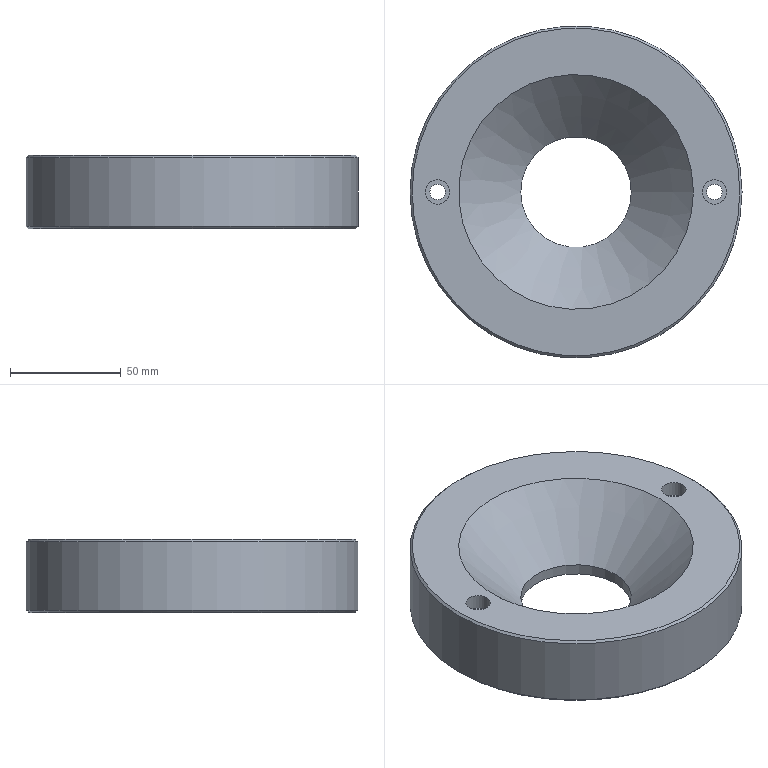Part | STEP file | 车灯-后视镜_id298_x_t | 1 solid | 13 faces | box 149.9 x 149.9 x 33 mm | volume 429222 mm3 | cylinder 6 | plane 4 | cone 3 | commonest cylinder face diameters 7 x2 11 x2 50 x1 149.9 x1
STEP:
#1=CARTESIAN_POINT('',(31.,-25.,243.5));
#2=VERTEX_POINT('',#1);
#3=CARTESIAN_POINT('',(-22.,-25.,243.5));
#4=DIRECTION('',(0.,0.,-1.));
#5=DIRECTION('',(1.,0.,0.));
#6=AXIS2_PLACEMENT_3D('',#3,#4,#5);
#7=CIRCLE('',#6,53.);
#8=EDGE_CURVE('',#2,#2,#7,.T.);
#9=ORIENTED_EDGE('',*,*,#8,.T.);
#10=EDGE_LOOP('',(#9));
#11=FACE_BOUND('',#10,.T.);
#12=CARTESIAN_POINT('',(51.95,-25.,243.5));
#13=VERTEX_POINT('',#12);
#14=CARTESIAN_POINT('',(-22.,-25.,243.5));
#15=DIRECTION('',(0.,0.,1.));
#16=DIRECTION('',(1.,0.,0.));
#17=AXIS2_PLACEMENT_3D('',#14,#15,#16);
#18=CIRCLE('',#17,73.95);
#19=EDGE_CURVE('',#13,#13,#18,.T.);
#20=ORIENTED_EDGE('',*,*,#19,.T.);
#21=EDGE_LOOP('',(#20));
#22=FACE_BOUND('',#21,.T.);
#23=CARTESIAN_POINT('',(46.,-25.,243.5));
#24=VERTEX_POINT('',#23);
#25=CARTESIAN_POINT('',(40.5,-25.,243.5));
#26=DIRECTION('',(0.,0.,1.));
#27=DIRECTION('',(1.,0.,0.));
#28=AXIS2_PLACEMENT_3D('',#25,#26,#27);
#29=CIRCLE('',#28,5.5);
#30=EDGE_CURVE('',#24,#24,#29,.T.);
#31=ORIENTED_EDGE('',*,*,#30,.F.);
#32=EDGE_LOOP('',(#31));
#33=FACE_BOUND('',#32,.T.);
#34=CARTESIAN_POINT('',(-79.,-25.,243.5));
#35=VERTEX_POINT('',#34);
#36=CARTESIAN_POINT('',(-84.5,-25.,243.5));
#37=DIRECTION('',(0.,0.,-1.));
#38=DIRECTION('',(1.,0.,0.));
#39=AXIS2_PLACEMENT_3D('',#36,#37,#38);
#40=CIRCLE('',#39,5.5);
#41=EDGE_CURVE('',#35,#35,#40,.T.);
#42=ORIENTED_EDGE('',*,*,#41,.T.);
#43=EDGE_LOOP('',(#42));
#44=FACE_BOUND('',#43,.T.);
#45=CARTESIAN_POINT('',(-22.,-25.,243.5));
#46=DIRECTION('',(0.,0.,1.));
#47=DIRECTION('',(0.,1.,0.));
#48=AXIS2_PLACEMENT_3D('',#45,#46,#47);
#49=PLANE('',#48);
#50=ADVANCED_FACE('',(#11,#22,#33,#44),#49,.T.);
#51=CARTESIAN_POINT('',(-95.95,-25.,210.5));
#52=VERTEX_POINT('',#51);
#53=CARTESIAN_POINT('',(-22.,-25.,210.5));
#54=DIRECTION('',(0.,0.,-1.));
#55=DIRECTION('',(-1.,0.,0.));
#56=AXIS2_PLACEMENT_3D('',#53,#54,#55);
#57=CIRCLE('',#56,73.95);
#58=EDGE_CURVE('',#52,#52,#57,.T.);
#59=ORIENTED_EDGE('',*,*,#58,.T.);
#60=EDGE_LOOP('',(#59));
#61=FACE_BOUND('',#60,.T.);
#62=CARTESIAN_POINT('',(37.,-25.,210.5));
#63=VERTEX_POINT('',#62);
#64=CARTESIAN_POINT('',(40.5,-25.,210.5));
#65=DIRECTION('',(0.,0.,-1.));
#66=DIRECTION('',(-1.,0.,0.));
#67=AXIS2_PLACEMENT_3D('',#64,#65,#66);
#68=CIRCLE('',#67,3.5);
#69=EDGE_CURVE('',#63,#63,#68,.T.);
#70=ORIENTED_EDGE('',*,*,#69,.F.);
#71=EDGE_LOOP('',(#70));
#72=FACE_BOUND('',#71,.T.);
#73=CARTESIAN_POINT('',(-88.,-25.,210.5));
#74=VERTEX_POINT('',#73);
#75=CARTESIAN_POINT('',(-84.5,-25.,210.5));
#76=DIRECTION('',(0.,0.,-1.));
#77=DIRECTION('',(-1.,0.,0.));
#78=AXIS2_PLACEMENT_3D('',#75,#76,#77);
#79=CIRCLE('',#78,3.5);
#80=EDGE_CURVE('',#74,#74,#79,.T.);
#81=ORIENTED_EDGE('',*,*,#80,.F.);
#82=EDGE_LOOP('',(#81));
#83=FACE_BOUND('',#82,.T.);
#84=CARTESIAN_POINT('',(-47.,-25.,210.5));
#85=VERTEX_POINT('',#84);
#86=CARTESIAN_POINT('',(-22.,-25.,210.5));
#87=DIRECTION('',(0.,0.,-1.));
#88=DIRECTION('',(-1.,0.,0.));
#89=AXIS2_PLACEMENT_3D('',#86,#87,#88);
#90=CIRCLE('',#89,25.);
#91=EDGE_CURVE('',#85,#85,#90,.T.);
#92=ORIENTED_EDGE('',*,*,#91,.F.);
#93=EDGE_LOOP('',(#92));
#94=FACE_BOUND('',#93,.T.);
#95=CARTESIAN_POINT('',(-22.,-25.,210.5));
#96=DIRECTION('',(0.,0.,-1.));
#97=DIRECTION('',(0.,-1.,0.));
#98=AXIS2_PLACEMENT_3D('',#95,#96,#97);
#99=PLANE('',#98);
#100=ADVANCED_FACE('',(#61,#72,#83,#94),#99,.T.);
#101=CARTESIAN_POINT('',(-96.95,-25.,242.5));
#102=VERTEX_POINT('',#101);
#103=CARTESIAN_POINT('',(-22.,-25.,242.5));
#104=DIRECTION('',(0.,0.,-1.));
#105=DIRECTION('',(-1.,0.,0.));
#106=AXIS2_PLACEMENT_3D('',#103,#104,#105);
#107=CIRCLE('',#106,74.95);
#108=EDGE_CURVE('',#102,#102,#107,.T.);
#109=ORIENTED_EDGE('',*,*,#108,.T.);
#110=EDGE_LOOP('',(#109));
#111=FACE_BOUND('',#110,.T.);
#112=CARTESIAN_POINT('',(-96.95,-25.,211.5));
#113=VERTEX_POINT('',#112);
#114=CARTESIAN_POINT('',(-22.,-25.,211.5));
#115=DIRECTION('',(0.,0.,1.));
#116=DIRECTION('',(-1.,0.,0.));
#117=AXIS2_PLACEMENT_3D('',#114,#115,#116);
#118=CIRCLE('',#117,74.95);
#119=EDGE_CURVE('',#113,#113,#118,.T.);
#120=ORIENTED_EDGE('',*,*,#119,.T.);
#121=EDGE_LOOP('',(#120));
#122=FACE_BOUND('',#121,.T.);
#123=CARTESIAN_POINT('',(-22.,-25.,210.5));
#124=DIRECTION('',(0.,0.,1.));
#125=DIRECTION('',(0.,1.,0.));
#126=AXIS2_PLACEMENT_3D('',#123,#124,#125);
#127=CYLINDRICAL_SURFACE('',#126,74.95);
#128=ADVANCED_FACE('',(#111,#122),#127,.T.);
#129=CARTESIAN_POINT('',(3.,-25.,215.5));
#130=VERTEX_POINT('',#129);
#131=CARTESIAN_POINT('',(-22.,-25.,215.5));
#132=DIRECTION('',(0.,0.,1.));
#133=DIRECTION('',(1.,0.,0.));
#134=AXIS2_PLACEMENT_3D('',#131,#132,#133);
#135=CIRCLE('',#134,25.);
#136=EDGE_CURVE('',#130,#130,#135,.T.);
#137=ORIENTED_EDGE('',*,*,#136,.T.);
#138=EDGE_LOOP('',(#137));
#139=FACE_BOUND('',#138,.T.);
#140=ORIENTED_EDGE('',*,*,#91,.T.);
#141=EDGE_LOOP('',(#140));
#142=FACE_BOUND('',#141,.T.);
#143=CARTESIAN_POINT('',(-22.,-25.,225.5));
#144=DIRECTION('',(0.,0.,-1.));
#145=DIRECTION('',(0.,-1.,0.));
#146=AXIS2_PLACEMENT_3D('',#143,#144,#145);
#147=CYLINDRICAL_SURFACE('',#146,25.);
#148=ADVANCED_FACE('',(#139,#142),#147,.F.);
#149=ORIENTED_EDGE('',*,*,#80,.T.);
#150=EDGE_LOOP('',(#149));
#151=FACE_BOUND('',#150,.T.);
#152=CARTESIAN_POINT('',(-88.,-25.,236.5));
#153=VERTEX_POINT('',#152);
#154=CARTESIAN_POINT('',(-84.5,-25.,236.5));
#155=DIRECTION('',(0.,0.,-1.));
#156=DIRECTION('',(-1.,0.,0.));
#157=AXIS2_PLACEMENT_3D('',#154,#155,#156);
#158=CIRCLE('',#157,3.5);
#159=EDGE_CURVE('',#153,#153,#158,.T.);
#160=ORIENTED_EDGE('',*,*,#159,.F.);
#161=EDGE_LOOP('',(#160));
#162=FACE_BOUND('',#161,.T.);
#163=CARTESIAN_POINT('',(-84.5,-25.,125.5));
#164=DIRECTION('',(0.,0.,-1.));
#165=DIRECTION('',(0.,-1.,0.));
#166=AXIS2_PLACEMENT_3D('',#163,#164,#165);
#167=CYLINDRICAL_SURFACE('',#166,3.5);
#168=ADVANCED_FACE('',(#151,#162),#167,.F.);
#169=ORIENTED_EDGE('',*,*,#159,.T.);
#170=EDGE_LOOP('',(#169));
#171=FACE_BOUND('',#170,.T.);
#172=CARTESIAN_POINT('',(-90.,-25.,236.5));
#173=VERTEX_POINT('',#172);
#174=CARTESIAN_POINT('',(-84.5,-25.,236.5));
#175=DIRECTION('',(0.,0.,-1.));
#176=DIRECTION('',(-1.,0.,0.));
#177=AXIS2_PLACEMENT_3D('',#174,#175,#176);
#178=CIRCLE('',#177,5.5);
#179=EDGE_CURVE('',#173,#173,#178,.T.);
#180=ORIENTED_EDGE('',*,*,#179,.F.);
#181=EDGE_LOOP('',(#180));
#182=FACE_BOUND('',#181,.T.);
#183=CARTESIAN_POINT('',(-84.5,-25.,236.5));
#184=DIRECTION('',(0.,0.,-1.));
#185=DIRECTION('',(0.,-1.,0.));
#186=AXIS2_PLACEMENT_3D('',#183,#184,#185);
#187=PLANE('',#186);
#188=ADVANCED_FACE('',(#171,#182),#187,.F.);
#189=ORIENTED_EDGE('',*,*,#179,.T.);
#190=EDGE_LOOP('',(#189));
#191=FACE_BOUND('',#190,.T.);
#192=ORIENTED_EDGE('',*,*,#41,.F.);
#193=EDGE_LOOP('',(#192));
#194=FACE_BOUND('',#193,.T.);
#195=CARTESIAN_POINT('',(-84.5,-25.,233.5));
#196=DIRECTION('',(0.,0.,-1.));
#197=DIRECTION('',(0.,-1.,0.));
#198=AXIS2_PLACEMENT_3D('',#195,#196,#197);
#199=CYLINDRICAL_SURFACE('',#198,5.5);
#200=ADVANCED_FACE('',(#191,#194),#199,.F.);
#201=ORIENTED_EDGE('',*,*,#69,.T.);
#202=EDGE_LOOP('',(#201));
#203=FACE_BOUND('',#202,.T.);
#204=CARTESIAN_POINT('',(37.,-25.,236.5));
#205=VERTEX_POINT('',#204);
#206=CARTESIAN_POINT('',(40.5,-25.,236.5));
#207=DIRECTION('',(0.,0.,1.));
#208=DIRECTION('',(-1.,0.,0.));
#209=AXIS2_PLACEMENT_3D('',#206,#207,#208);
#210=CIRCLE('',#209,3.5);
#211=EDGE_CURVE('',#205,#205,#210,.T.);
#212=ORIENTED_EDGE('',*,*,#211,.T.);
#213=EDGE_LOOP('',(#212));
#214=FACE_BOUND('',#213,.T.);
#215=CARTESIAN_POINT('',(40.5,-25.,125.5));
#216=DIRECTION('',(0.,0.,-1.));
#217=DIRECTION('',(0.,-1.,0.));
#218=AXIS2_PLACEMENT_3D('',#215,#216,#217);
#219=CYLINDRICAL_SURFACE('',#218,3.5);
#220=ADVANCED_FACE('',(#203,#214),#219,.F.);
#221=ORIENTED_EDGE('',*,*,#211,.F.);
#222=EDGE_LOOP('',(#221));
#223=FACE_BOUND('',#222,.T.);
#224=CARTESIAN_POINT('',(35.,-25.,236.5));
#225=VERTEX_POINT('',#224);
#226=CARTESIAN_POINT('',(40.5,-25.,236.5));
#227=DIRECTION('',(0.,0.,1.));
#228=DIRECTION('',(-1.,0.,0.));
#229=AXIS2_PLACEMENT_3D('',#226,#227,#228);
#230=CIRCLE('',#229,5.5);
#231=EDGE_CURVE('',#225,#225,#230,.T.);
#232=ORIENTED_EDGE('',*,*,#231,.T.);
#233=EDGE_LOOP('',(#232));
#234=FACE_BOUND('',#233,.T.);
#235=CARTESIAN_POINT('',(40.5,-25.,236.5));
#236=DIRECTION('',(0.,0.,-1.));
#237=DIRECTION('',(0.,-1.,0.));
#238=AXIS2_PLACEMENT_3D('',#235,#236,#237);
#239=PLANE('',#238);
#240=ADVANCED_FACE('',(#223,#234),#239,.F.);
#241=ORIENTED_EDGE('',*,*,#231,.F.);
#242=EDGE_LOOP('',(#241));
#243=FACE_BOUND('',#242,.T.);
#244=ORIENTED_EDGE('',*,*,#30,.T.);
#245=EDGE_LOOP('',(#244));
#246=FACE_BOUND('',#245,.T.);
#247=CARTESIAN_POINT('',(40.5,-25.,233.5));
#248=DIRECTION('',(0.,0.,-1.));
#249=DIRECTION('',(0.,-1.,0.));
#250=AXIS2_PLACEMENT_3D('',#247,#248,#249);
#251=CYLINDRICAL_SURFACE('',#250,5.5);
#252=ADVANCED_FACE('',(#243,#246),#251,.F.);
#253=ORIENTED_EDGE('',*,*,#108,.F.);
#254=EDGE_LOOP('',(#253));
#255=FACE_BOUND('',#254,.T.);
#256=ORIENTED_EDGE('',*,*,#19,.F.);
#257=EDGE_LOOP('',(#256));
#258=FACE_BOUND('',#257,.T.);
#259=CARTESIAN_POINT('',(-22.,-25.,243.5));
#260=DIRECTION('',(0.,0.,-1.));
#261=DIRECTION('',(-1.,0.,0.));
#262=AXIS2_PLACEMENT_3D('',#259,#260,#261);
#263=CONICAL_SURFACE('',#262,73.95,45.);
#264=ADVANCED_FACE('',(#255,#258),#263,.T.);
#265=ORIENTED_EDGE('',*,*,#119,.F.);
#266=EDGE_LOOP('',(#265));
#267=FACE_BOUND('',#266,.T.);
#268=ORIENTED_EDGE('',*,*,#58,.F.);
#269=EDGE_LOOP('',(#268));
#270=FACE_BOUND('',#269,.T.);
#271=CARTESIAN_POINT('',(-22.,-25.,210.5));
#272=DIRECTION('',(0.,0.,1.));
#273=DIRECTION('',(1.,0.,0.));
#274=AXIS2_PLACEMENT_3D('',#271,#272,#273);
#275=CONICAL_SURFACE('',#274,73.95,45.);
#276=ADVANCED_FACE('',(#267,#270),#275,.T.);
#277=ORIENTED_EDGE('',*,*,#136,.F.);
#278=EDGE_LOOP('',(#277));
#279=FACE_BOUND('',#278,.T.);
#280=ORIENTED_EDGE('',*,*,#8,.F.);
#281=EDGE_LOOP('',(#280));
#282=FACE_BOUND('',#281,.T.);
#283=CARTESIAN_POINT('',(-22.,-25.,243.5));
#284=DIRECTION('',(0.,0.,1.));
#285=DIRECTION('',(1.,0.,0.));
#286=AXIS2_PLACEMENT_3D('',#283,#284,#285);
#287=CONICAL_SURFACE('',#286,53.,45.);
#288=ADVANCED_FACE('',(#279,#282),#287,.F.);
#289=CLOSED_SHELL('',(#50,#100,#128,#148,#168,#188,#200,#220,#240,#252,#264,#276,#288));
#290=MANIFOLD_SOLID_BREP('',#289);
#291=(LENGTH_UNIT()NAMED_UNIT(*)SI_UNIT(.MILLI.,.METRE.));
#292=UNCERTAINTY_MEASURE_WITH_UNIT(LENGTH_MEASURE(0.00002),#291,'','');
#293=(NAMED_UNIT(*)PLANE_ANGLE_UNIT()SI_UNIT($,.RADIAN.));
#294=PLANE_ANGLE_MEASURE_WITH_UNIT(PLANE_ANGLE_MEASURE(0.01745),#293);
#295=DIMENSIONAL_EXPONENTS(0.,0.,0.,0.,0.,0.,0.);
#296=(CONVERSION_BASED_UNIT('DEGREE',#294)NAMED_UNIT(#295)PLANE_ANGLE_UNIT());
#297=(NAMED_UNIT(*)SI_UNIT($,.STERADIAN.)SOLID_ANGLE_UNIT());
#298=(GEOMETRIC_REPRESENTATION_CONTEXT(3)GLOBAL_UNCERTAINTY_ASSIGNED_CONTEXT((#292))GLOBAL_UNIT_ASSIGNED_CONTEXT((#291,#296,#297))REPRESENTATION_CONTEXT('',''));
#299=ADVANCED_BREP_SHAPE_REPRESENTATION('',(#290),#298);